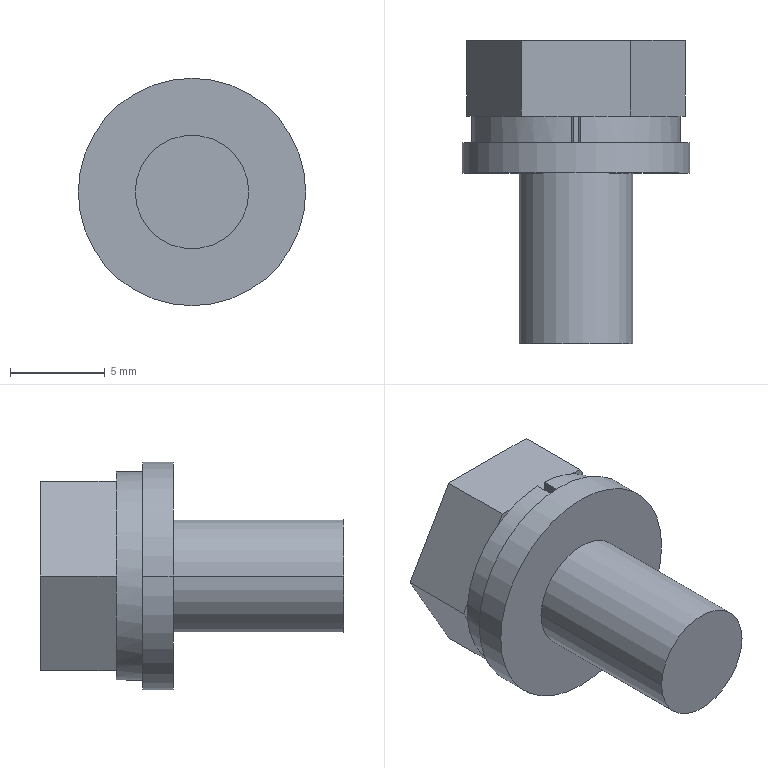Part | STEP file | LIB_36623101_M6X12 | 1 solid | 45 faces | box 12 x 16 x 12 mm | volume 879.589 mm3 | plane 27 | cylinder 18 | commonest cylinder face diameters 0.809 x6 2 x6 6 x3 12 x2 11 x1